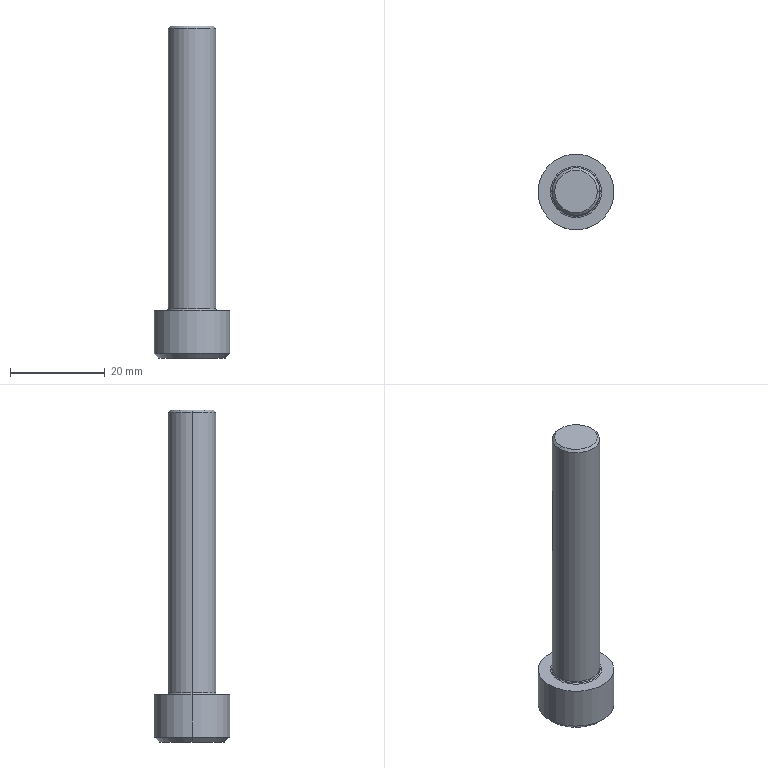Part | Creo | 1 solid | 23 faces | box 16 x 16 x 70 mm | volume 6361 mm3 | plane 9 | cone 6 | cylinder 4 | torus 4 | commonest cylinder face diameters 10 x2 16 x2
STEP:
#1=CARTESIAN_POINT('',(-135.619,-45.005,39.5));
#2=VERTEX_POINT('',#1);
#3=CARTESIAN_POINT('',(-133.309,-41.005,39.5));
#4=VERTEX_POINT('',#3);
#5=CARTESIAN_POINT('',(-135.619,-45.005,39.5));
#6=CARTESIAN_POINT('',(-135.493,-44.787,39.573));
#7=CARTESIAN_POINT('',(-135.241,-44.35,39.701));
#8=CARTESIAN_POINT('',(-134.855,-43.682,39.827));
#9=CARTESIAN_POINT('',(-134.465,-43.007,39.872));
#10=CARTESIAN_POINT('',(-134.074,-42.329,39.828));
#11=CARTESIAN_POINT('',(-133.689,-41.662,39.701));
#12=CARTESIAN_POINT('',(-133.436,-41.223,39.573));
#13=CARTESIAN_POINT('',(-133.309,-41.005,39.5));
#14=B_SPLINE_CURVE_WITH_KNOTS('',3,(#5,#6,#7,#8,#9,#10,#11,#12,#13),.UNSPECIFIED.,.F.,.F.,(4,1,1,1,1,1,4),(0.,0.1667,0.3333,0.5,0.6667,0.8333,1.),.UNSPECIFIED.);
#15=EDGE_CURVE('',#2,#4,#14,.T.);
#16=ORIENTED_EDGE('',*,*,#15,.F.);
#17=CARTESIAN_POINT('',(-131.,-45.005,42.167));
#18=VERTEX_POINT('',#17);
#19=CARTESIAN_POINT('',(-131.,-45.005,42.167));
#20=DIRECTION('',(-0.866,0.,-0.5));
#21=VECTOR('',#20,5.333);
#22=LINE('',#19,#21);
#23=EDGE_CURVE('',#18,#2,#22,.T.);
#24=ORIENTED_EDGE('',*,*,#23,.F.);
#25=CARTESIAN_POINT('',(-126.381,-45.005,39.5));
#26=VERTEX_POINT('',#25);
#27=CARTESIAN_POINT('',(-131.,-45.005,42.167));
#28=DIRECTION('',(0.866,0.,-0.5));
#29=VECTOR('',#28,5.333);
#30=LINE('',#27,#29);
#31=EDGE_CURVE('',#18,#26,#30,.T.);
#32=ORIENTED_EDGE('',*,*,#31,.T.);
#33=CARTESIAN_POINT('',(-128.691,-41.005,39.5));
#34=VERTEX_POINT('',#33);
#35=CARTESIAN_POINT('',(-128.691,-41.005,39.5));
#36=CARTESIAN_POINT('',(-128.565,-41.222,39.573));
#37=CARTESIAN_POINT('',(-128.313,-41.659,39.701));
#38=CARTESIAN_POINT('',(-127.927,-42.328,39.827));
#39=CARTESIAN_POINT('',(-127.537,-43.003,39.872));
#40=CARTESIAN_POINT('',(-127.146,-43.68,39.828));
#41=CARTESIAN_POINT('',(-126.761,-44.348,39.701));
#42=CARTESIAN_POINT('',(-126.507,-44.786,39.573));
#43=CARTESIAN_POINT('',(-126.381,-45.005,39.5));
#44=B_SPLINE_CURVE_WITH_KNOTS('',3,(#35,#36,#37,#38,#39,#40,#41,#42,#43),.UNSPECIFIED.,.F.,.F.,(4,1,1,1,1,1,4),(0.,0.1667,0.3333,0.5,0.6667,0.8333,1.),.UNSPECIFIED.);
#45=EDGE_CURVE('',#34,#26,#44,.T.);
#46=ORIENTED_EDGE('',*,*,#45,.F.);
#47=CARTESIAN_POINT('',(-133.309,-41.005,39.5));
#48=CARTESIAN_POINT('',(-133.059,-41.005,39.572));
#49=CARTESIAN_POINT('',(-132.556,-41.005,39.7));
#50=CARTESIAN_POINT('',(-131.782,-41.005,39.827));
#51=CARTESIAN_POINT('',(-131.001,-41.005,39.872));
#52=CARTESIAN_POINT('',(-130.221,-41.005,39.828));
#53=CARTESIAN_POINT('',(-129.447,-41.005,39.701));
#54=CARTESIAN_POINT('',(-128.942,-41.005,39.573));
#55=CARTESIAN_POINT('',(-128.691,-41.005,39.5));
#56=B_SPLINE_CURVE_WITH_KNOTS('',3,(#47,#48,#49,#50,#51,#52,#53,#54,#55),.UNSPECIFIED.,.F.,.F.,(4,1,1,1,1,1,4),(0.,0.1667,0.3333,0.5,0.6667,0.8333,1.),.UNSPECIFIED.);
#57=EDGE_CURVE('',#4,#34,#56,.T.);
#58=ORIENTED_EDGE('',*,*,#57,.F.);
#59=EDGE_LOOP('',(#16,#24,#32,#46,#58));
#60=FACE_OUTER_BOUND('',#59,.F.);
#61=CARTESIAN_POINT('',(-131.,-45.005,40.807));
#62=DIRECTION('',(0.,0.,-1.));
#63=DIRECTION('',(-1.,0.,0.));
#64=AXIS2_PLACEMENT_3D('',#61,#62,#63);
#65=CONICAL_SURFACE('',#64,2.356,60.);
#66=ADVANCED_FACE('',(#60),#65,.F.);
#67=CARTESIAN_POINT('',(-133.309,-41.005,34.5));
#68=VERTEX_POINT('',#67);
#69=CARTESIAN_POINT('',(-135.619,-45.005,34.5));
#70=VERTEX_POINT('',#69);
#71=CARTESIAN_POINT('',(-133.309,-41.005,34.5));
#72=DIRECTION('',(-0.5,-0.866,0.));
#73=VECTOR('',#72,4.619);
#74=LINE('',#71,#73);
#75=EDGE_CURVE('',#68,#70,#74,.T.);
#76=ORIENTED_EDGE('',*,*,#75,.T.);
#77=CARTESIAN_POINT('',(-135.619,-45.005,34.5));
#78=DIRECTION('',(0.,0.,1.));
#79=VECTOR('',#78,5.);
#80=LINE('',#77,#79);
#81=EDGE_CURVE('',#70,#2,#80,.T.);
#82=ORIENTED_EDGE('',*,*,#81,.T.);
#83=ORIENTED_EDGE('',*,*,#15,.T.);
#84=CARTESIAN_POINT('',(-133.309,-41.005,34.5));
#85=DIRECTION('',(0.,0.,1.));
#86=VECTOR('',#85,5.);
#87=LINE('',#84,#86);
#88=EDGE_CURVE('',#68,#4,#87,.T.);
#89=ORIENTED_EDGE('',*,*,#88,.F.);
#90=EDGE_LOOP('',(#76,#82,#83,#89));
#91=FACE_OUTER_BOUND('',#90,.F.);
#92=CARTESIAN_POINT('',(-133.309,-41.005,39.5));
#93=DIRECTION('',(0.866,-0.5,0.));
#94=DIRECTION('',(-0.5,-0.866,0.));
#95=AXIS2_PLACEMENT_3D('',#92,#93,#94);
#96=PLANE('',#95);
#97=ADVANCED_FACE('',(#91),#96,.T.);
#98=CARTESIAN_POINT('',(-138.,-45.005,34.5));
#99=VERTEX_POINT('',#98);
#100=CARTESIAN_POINT('',(-124.,-45.005,34.5));
#101=VERTEX_POINT('',#100);
#102=CARTESIAN_POINT('',(-131.,-45.005,34.5));
#103=DIRECTION('',(0.,0.,-1.));
#104=DIRECTION('',(-1.,0.,0.));
#105=AXIS2_PLACEMENT_3D('',#102,#103,#104);
#106=CIRCLE('',#105,7.);
#107=EDGE_CURVE('',#99,#101,#106,.T.);
#108=ORIENTED_EDGE('',*,*,#107,.F.);
#109=CARTESIAN_POINT('',(-131.,-45.005,34.5));
#110=DIRECTION('',(0.,0.,-1.));
#111=DIRECTION('',(1.,0.,0.));
#112=AXIS2_PLACEMENT_3D('',#109,#110,#111);
#113=CIRCLE('',#112,7.);
#114=EDGE_CURVE('',#101,#99,#113,.T.);
#115=ORIENTED_EDGE('',*,*,#114,.F.);
#116=EDGE_LOOP('',(#108,#115));
#117=FACE_OUTER_BOUND('',#116,.F.);
#118=CARTESIAN_POINT('',(-133.309,-49.005,34.5));
#119=VERTEX_POINT('',#118);
#120=CARTESIAN_POINT('',(-135.619,-45.005,34.5));
#121=DIRECTION('',(0.5,-0.866,0.));
#122=VECTOR('',#121,4.619);
#123=LINE('',#120,#122);
#124=EDGE_CURVE('',#70,#119,#123,.T.);
#125=ORIENTED_EDGE('',*,*,#124,.F.);
#126=ORIENTED_EDGE('',*,*,#75,.F.);
#127=CARTESIAN_POINT('',(-128.691,-41.005,34.5));
#128=VERTEX_POINT('',#127);
#129=CARTESIAN_POINT('',(-133.309,-41.005,34.5));
#130=DIRECTION('',(1.,0.,0.));
#131=VECTOR('',#130,4.619);
#132=LINE('',#129,#131);
#133=EDGE_CURVE('',#68,#128,#132,.T.);
#134=ORIENTED_EDGE('',*,*,#133,.T.);
#135=CARTESIAN_POINT('',(-126.381,-45.005,34.5));
#136=VERTEX_POINT('',#135);
#137=CARTESIAN_POINT('',(-126.381,-45.005,34.5));
#138=DIRECTION('',(-0.5,0.866,0.));
#139=VECTOR('',#138,4.619);
#140=LINE('',#137,#139);
#141=EDGE_CURVE('',#136,#128,#140,.T.);
#142=ORIENTED_EDGE('',*,*,#141,.F.);
#143=CARTESIAN_POINT('',(-128.691,-49.005,34.5));
#144=VERTEX_POINT('',#143);
#145=CARTESIAN_POINT('',(-128.691,-49.005,34.5));
#146=DIRECTION('',(0.5,0.866,0.));
#147=VECTOR('',#146,4.619);
#148=LINE('',#145,#147);
#149=EDGE_CURVE('',#144,#136,#148,.T.);
#150=ORIENTED_EDGE('',*,*,#149,.F.);
#151=CARTESIAN_POINT('',(-128.691,-49.005,34.5));
#152=DIRECTION('',(-1.,0.,0.));
#153=VECTOR('',#152,4.619);
#154=LINE('',#151,#153);
#155=EDGE_CURVE('',#144,#119,#154,.T.);
#156=ORIENTED_EDGE('',*,*,#155,.T.);
#157=EDGE_LOOP('',(#125,#126,#134,#142,#150,#156));
#158=FACE_BOUND('',#157,.F.);
#159=CARTESIAN_POINT('',(-131.,-45.005,34.5));
#160=DIRECTION('',(0.,0.,-1.));
#161=DIRECTION('',(-1.,0.,0.));
#162=AXIS2_PLACEMENT_3D('',#159,#160,#161);
#163=PLANE('',#162);
#164=ADVANCED_FACE('',(#117,#158),#163,.T.);
#165=CARTESIAN_POINT('',(-139.,-45.005,35.5));
#166=VERTEX_POINT('',#165);
#167=CARTESIAN_POINT('',(-123.,-45.005,35.5));
#168=VERTEX_POINT('',#167);
#169=CARTESIAN_POINT('',(-131.,-45.005,35.5));
#170=DIRECTION('',(0.,0.,-1.));
#171=DIRECTION('',(-1.,0.,0.));
#172=AXIS2_PLACEMENT_3D('',#169,#170,#171);
#173=CIRCLE('',#172,8.);
#174=EDGE_CURVE('',#166,#168,#173,.T.);
#175=ORIENTED_EDGE('',*,*,#174,.F.);
#176=CARTESIAN_POINT('',(-138.,-45.005,34.5));
#177=DIRECTION('',(-0.7071,0.,0.7071));
#178=VECTOR('',#177,1.414);
#179=LINE('',#176,#178);
#180=EDGE_CURVE('',#99,#166,#179,.T.);
#181=ORIENTED_EDGE('',*,*,#180,.F.);
#182=ORIENTED_EDGE('',*,*,#107,.T.);
#183=CARTESIAN_POINT('',(-124.,-45.005,34.5));
#184=DIRECTION('',(0.7071,0.,0.7071));
#185=VECTOR('',#184,1.414);
#186=LINE('',#183,#185);
#187=EDGE_CURVE('',#101,#168,#186,.T.);
#188=ORIENTED_EDGE('',*,*,#187,.T.);
#189=EDGE_LOOP('',(#175,#181,#182,#188));
#190=FACE_OUTER_BOUND('',#189,.F.);
#191=CARTESIAN_POINT('',(-131.,-45.005,35.));
#192=DIRECTION('',(0.,0.,1.));
#193=DIRECTION('',(1.,0.,0.));
#194=AXIS2_PLACEMENT_3D('',#191,#192,#193);
#195=CONICAL_SURFACE('',#194,7.5,45.);
#196=ADVANCED_FACE('',(#190),#195,.T.);
#197=ORIENTED_EDGE('',*,*,#174,.T.);
#198=CARTESIAN_POINT('',(-123.,-45.005,44.5));
#199=VERTEX_POINT('',#198);
#200=CARTESIAN_POINT('',(-123.,-45.005,44.5));
#201=DIRECTION('',(0.,0.,-1.));
#202=VECTOR('',#201,9.);
#203=LINE('',#200,#202);
#204=EDGE_CURVE('',#199,#168,#203,.T.);
#205=ORIENTED_EDGE('',*,*,#204,.F.);
#206=CARTESIAN_POINT('',(-139.,-45.005,44.5));
#207=VERTEX_POINT('',#206);
#208=CARTESIAN_POINT('',(-131.,-45.005,44.5));
#209=DIRECTION('',(0.,0.,1.));
#210=DIRECTION('',(1.,0.,0.));
#211=AXIS2_PLACEMENT_3D('',#208,#209,#210);
#212=CIRCLE('',#211,8.);
#213=EDGE_CURVE('',#199,#207,#212,.T.);
#214=ORIENTED_EDGE('',*,*,#213,.T.);
#215=CARTESIAN_POINT('',(-139.,-45.005,44.5));
#216=DIRECTION('',(0.,0.,-1.));
#217=VECTOR('',#216,9.);
#218=LINE('',#215,#217);
#219=EDGE_CURVE('',#207,#166,#218,.T.);
#220=ORIENTED_EDGE('',*,*,#219,.T.);
#221=EDGE_LOOP('',(#197,#205,#214,#220));
#222=FACE_OUTER_BOUND('',#221,.F.);
#223=CARTESIAN_POINT('',(-131.,-45.005,44.5));
#224=DIRECTION('',(0.,0.,-1.));
#225=DIRECTION('',(-1.,0.,0.));
#226=AXIS2_PLACEMENT_3D('',#223,#224,#225);
#227=CYLINDRICAL_SURFACE('',#226,8.);
#228=ADVANCED_FACE('',(#222),#227,.T.);
#229=CARTESIAN_POINT('',(-131.,-45.005,35.5));
#230=DIRECTION('',(0.,0.,-1.));
#231=DIRECTION('',(1.,0.,0.));
#232=AXIS2_PLACEMENT_3D('',#229,#230,#231);
#233=CIRCLE('',#232,8.);
#234=EDGE_CURVE('',#168,#166,#233,.T.);
#235=ORIENTED_EDGE('',*,*,#234,.T.);
#236=ORIENTED_EDGE('',*,*,#219,.F.);
#237=CARTESIAN_POINT('',(-131.,-45.005,44.5));
#238=DIRECTION('',(0.,0.,1.));
#239=DIRECTION('',(-1.,0.,0.));
#240=AXIS2_PLACEMENT_3D('',#237,#238,#239);
#241=CIRCLE('',#240,8.);
#242=EDGE_CURVE('',#207,#199,#241,.T.);
#243=ORIENTED_EDGE('',*,*,#242,.T.);
#244=ORIENTED_EDGE('',*,*,#204,.T.);
#245=EDGE_LOOP('',(#235,#236,#243,#244));
#246=FACE_OUTER_BOUND('',#245,.F.);
#247=CARTESIAN_POINT('',(-131.,-45.005,44.5));
#248=DIRECTION('',(0.,0.,-1.));
#249=DIRECTION('',(-1.,0.,0.));
#250=AXIS2_PLACEMENT_3D('',#247,#248,#249);
#251=CYLINDRICAL_SURFACE('',#250,8.);
#252=ADVANCED_FACE('',(#246),#251,.T.);
#253=ORIENTED_EDGE('',*,*,#234,.F.);
#254=ORIENTED_EDGE('',*,*,#187,.F.);
#255=ORIENTED_EDGE('',*,*,#114,.T.);
#256=ORIENTED_EDGE('',*,*,#180,.T.);
#257=EDGE_LOOP('',(#253,#254,#255,#256));
#258=FACE_OUTER_BOUND('',#257,.F.);
#259=CARTESIAN_POINT('',(-131.,-45.005,35.));
#260=DIRECTION('',(0.,0.,1.));
#261=DIRECTION('',(1.,0.,0.));
#262=AXIS2_PLACEMENT_3D('',#259,#260,#261);
#263=CONICAL_SURFACE('',#262,7.5,45.);
#264=ADVANCED_FACE('',(#258),#263,.T.);
#265=ORIENTED_EDGE('',*,*,#242,.F.);
#266=ORIENTED_EDGE('',*,*,#213,.F.);
#267=EDGE_LOOP('',(#265,#266));
#268=FACE_OUTER_BOUND('',#267,.F.);
#269=CARTESIAN_POINT('',(-136.4,-45.005,44.5));
#270=VERTEX_POINT('',#269);
#271=CARTESIAN_POINT('',(-125.6,-45.005,44.5));
#272=VERTEX_POINT('',#271);
#273=CARTESIAN_POINT('',(-131.,-45.005,44.5));
#274=DIRECTION('',(0.,0.,-1.));
#275=DIRECTION('',(-1.,0.,0.));
#276=AXIS2_PLACEMENT_3D('',#273,#274,#275);
#277=CIRCLE('',#276,5.4);
#278=EDGE_CURVE('',#270,#272,#277,.T.);
#279=ORIENTED_EDGE('',*,*,#278,.F.);
#280=CARTESIAN_POINT('',(-131.,-45.005,44.5));
#281=DIRECTION('',(0.,0.,-1.));
#282=DIRECTION('',(1.,0.,0.));
#283=AXIS2_PLACEMENT_3D('',#280,#281,#282);
#284=CIRCLE('',#283,5.4);
#285=EDGE_CURVE('',#272,#270,#284,.T.);
#286=ORIENTED_EDGE('',*,*,#285,.F.);
#287=EDGE_LOOP('',(#279,#286));
#288=FACE_BOUND('',#287,.F.);
#289=CARTESIAN_POINT('',(-131.,-45.005,44.5));
#290=DIRECTION('',(0.,0.,-1.));
#291=DIRECTION('',(-1.,0.,0.));
#292=AXIS2_PLACEMENT_3D('',#289,#290,#291);
#293=PLANE('',#292);
#294=ADVANCED_FACE('',(#268,#288),#293,.F.);
#295=ORIENTED_EDGE('',*,*,#278,.T.);
#296=CARTESIAN_POINT('',(-125.883,-45.005,44.617));
#297=VERTEX_POINT('',#296);
#298=CARTESIAN_POINT('',(-125.6,-45.005,44.9));
#299=DIRECTION('',(0.,1.,0.));
#300=DIRECTION('',(0.,0.,-1.));
#301=AXIS2_PLACEMENT_3D('',#298,#299,#300);
#302=CIRCLE('',#301,0.4);
#303=EDGE_CURVE('',#272,#297,#302,.T.);
#304=ORIENTED_EDGE('',*,*,#303,.T.);
#305=CARTESIAN_POINT('',(-136.117,-45.005,44.617));
#306=VERTEX_POINT('',#305);
#307=CARTESIAN_POINT('',(-131.,-45.005,44.617));
#308=DIRECTION('',(0.,0.,-1.));
#309=DIRECTION('',(-1.,0.,0.));
#310=AXIS2_PLACEMENT_3D('',#307,#308,#309);
#311=CIRCLE('',#310,5.117);
#312=EDGE_CURVE('',#306,#297,#311,.T.);
#313=ORIENTED_EDGE('',*,*,#312,.F.);
#314=CARTESIAN_POINT('',(-136.4,-45.005,44.9));
#315=DIRECTION('',(0.,-1.,0.));
#316=DIRECTION('',(0.,0.,-1.));
#317=AXIS2_PLACEMENT_3D('',#314,#315,#316);
#318=CIRCLE('',#317,0.4);
#319=EDGE_CURVE('',#270,#306,#318,.T.);
#320=ORIENTED_EDGE('',*,*,#319,.F.);
#321=EDGE_LOOP('',(#295,#304,#313,#320));
#322=FACE_OUTER_BOUND('',#321,.F.);
#323=CARTESIAN_POINT('',(-131.,-45.005,44.9));
#324=DIRECTION('',(0.,0.,-1.));
#325=DIRECTION('',(-1.,0.,0.));
#326=AXIS2_PLACEMENT_3D('',#323,#324,#325);
#327=TOROIDAL_SURFACE('',#326,5.4,0.4);
#328=ADVANCED_FACE('',(#322),#327,.F.);
#329=ORIENTED_EDGE('',*,*,#285,.T.);
#330=ORIENTED_EDGE('',*,*,#319,.T.);
#331=CARTESIAN_POINT('',(-131.,-45.005,44.617));
#332=DIRECTION('',(0.,0.,-1.));
#333=DIRECTION('',(1.,0.,0.));
#334=AXIS2_PLACEMENT_3D('',#331,#332,#333);
#335=CIRCLE('',#334,5.117);
#336=EDGE_CURVE('',#297,#306,#335,.T.);
#337=ORIENTED_EDGE('',*,*,#336,.F.);
#338=ORIENTED_EDGE('',*,*,#303,.F.);
#339=EDGE_LOOP('',(#329,#330,#337,#338));
#340=FACE_OUTER_BOUND('',#339,.F.);
#341=CARTESIAN_POINT('',(-131.,-45.005,44.9));
#342=DIRECTION('',(0.,0.,-1.));
#343=DIRECTION('',(-1.,0.,0.));
#344=AXIS2_PLACEMENT_3D('',#341,#342,#343);
#345=TOROIDAL_SURFACE('',#344,5.4,0.4);
#346=ADVANCED_FACE('',(#340),#345,.F.);
#347=CARTESIAN_POINT('',(-126.,-45.005,44.9));
#348=VERTEX_POINT('',#347);
#349=CARTESIAN_POINT('',(-136.,-45.005,44.9));
#350=VERTEX_POINT('',#349);
#351=CARTESIAN_POINT('',(-131.,-45.005,44.9));
#352=DIRECTION('',(0.,0.,-1.));
#353=DIRECTION('',(1.,0.,0.));
#354=AXIS2_PLACEMENT_3D('',#351,#352,#353);
#355=CIRCLE('',#354,5.);
#356=EDGE_CURVE('',#348,#350,#355,.T.);
#357=ORIENTED_EDGE('',*,*,#356,.F.);
#358=CARTESIAN_POINT('',(-125.6,-45.005,44.9));
#359=DIRECTION('',(0.,1.,0.));
#360=DIRECTION('',(-0.7071,0.,-0.7071));
#361=AXIS2_PLACEMENT_3D('',#358,#359,#360);
#362=CIRCLE('',#361,0.4);
#363=EDGE_CURVE('',#297,#348,#362,.T.);
#364=ORIENTED_EDGE('',*,*,#363,.F.);
#365=ORIENTED_EDGE('',*,*,#336,.T.);
#366=CARTESIAN_POINT('',(-136.4,-45.005,44.9));
#367=DIRECTION('',(0.,-1.,0.));
#368=DIRECTION('',(0.7071,0.,-0.7071));
#369=AXIS2_PLACEMENT_3D('',#366,#367,#368);
#370=CIRCLE('',#369,0.4);
#371=EDGE_CURVE('',#306,#350,#370,.T.);
#372=ORIENTED_EDGE('',*,*,#371,.T.);
#373=EDGE_LOOP('',(#357,#364,#365,#372));
#374=FACE_OUTER_BOUND('',#373,.F.);
#375=CARTESIAN_POINT('',(-131.,-45.005,44.9));
#376=DIRECTION('',(0.,0.,-1.));
#377=DIRECTION('',(-1.,0.,0.));
#378=AXIS2_PLACEMENT_3D('',#375,#376,#377);
#379=TOROIDAL_SURFACE('',#378,5.4,0.4);
#380=ADVANCED_FACE('',(#374),#379,.F.);
#381=CARTESIAN_POINT('',(-136.,-45.005,104.));
#382=VERTEX_POINT('',#381);
#383=CARTESIAN_POINT('',(-126.,-45.005,104.));
#384=VERTEX_POINT('',#383);
#385=CARTESIAN_POINT('',(-131.,-45.005,104.));
#386=DIRECTION('',(0.,0.,1.));
#387=DIRECTION('',(-1.,0.,0.));
#388=AXIS2_PLACEMENT_3D('',#385,#386,#387);
#389=CIRCLE('',#388,5.);
#390=EDGE_CURVE('',#382,#384,#389,.T.);
#391=ORIENTED_EDGE('',*,*,#390,.T.);
#392=CARTESIAN_POINT('',(-126.,-45.005,104.));
#393=DIRECTION('',(0.,0.,-1.));
#394=VECTOR('',#393,59.1);
#395=LINE('',#392,#394);
#396=EDGE_CURVE('',#384,#348,#395,.T.);
#397=ORIENTED_EDGE('',*,*,#396,.T.);
#398=ORIENTED_EDGE('',*,*,#356,.T.);
#399=CARTESIAN_POINT('',(-136.,-45.005,104.));
#400=DIRECTION('',(0.,0.,-1.));
#401=VECTOR('',#400,59.1);
#402=LINE('',#399,#401);
#403=EDGE_CURVE('',#382,#350,#402,.T.);
#404=ORIENTED_EDGE('',*,*,#403,.F.);
#405=EDGE_LOOP('',(#391,#397,#398,#404));
#406=FACE_OUTER_BOUND('',#405,.F.);
#407=CARTESIAN_POINT('',(-131.,-45.005,104.5));
#408=DIRECTION('',(0.,0.,-1.));
#409=DIRECTION('',(-1.,0.,0.));
#410=AXIS2_PLACEMENT_3D('',#407,#408,#409);
#411=CYLINDRICAL_SURFACE('',#410,5.);
#412=ADVANCED_FACE('',(#406),#411,.T.);
#413=CARTESIAN_POINT('',(-135.5,-45.005,104.5));
#414=VERTEX_POINT('',#413);
#415=CARTESIAN_POINT('',(-126.5,-45.005,104.5));
#416=VERTEX_POINT('',#415);
#417=CARTESIAN_POINT('',(-131.,-45.005,104.5));
#418=DIRECTION('',(0.,0.,1.));
#419=DIRECTION('',(-1.,0.,0.));
#420=AXIS2_PLACEMENT_3D('',#417,#418,#419);
#421=CIRCLE('',#420,4.5);
#422=EDGE_CURVE('',#414,#416,#421,.T.);
#423=ORIENTED_EDGE('',*,*,#422,.T.);
#424=CARTESIAN_POINT('',(-126.5,-45.005,104.5));
#425=DIRECTION('',(0.7071,0.,-0.7071));
#426=VECTOR('',#425,0.7071);
#427=LINE('',#424,#426);
#428=EDGE_CURVE('',#416,#384,#427,.T.);
#429=ORIENTED_EDGE('',*,*,#428,.T.);
#430=ORIENTED_EDGE('',*,*,#390,.F.);
#431=CARTESIAN_POINT('',(-135.5,-45.005,104.5));
#432=DIRECTION('',(-0.7071,0.,-0.7071));
#433=VECTOR('',#432,0.7071);
#434=LINE('',#431,#433);
#435=EDGE_CURVE('',#414,#382,#434,.T.);
#436=ORIENTED_EDGE('',*,*,#435,.F.);
#437=EDGE_LOOP('',(#423,#429,#430,#436));
#438=FACE_OUTER_BOUND('',#437,.F.);
#439=CARTESIAN_POINT('',(-131.,-45.005,104.25));
#440=DIRECTION('',(0.,0.,-1.));
#441=DIRECTION('',(-1.,0.,0.));
#442=AXIS2_PLACEMENT_3D('',#439,#440,#441);
#443=CONICAL_SURFACE('',#442,4.75,45.);
#444=ADVANCED_FACE('',(#438),#443,.T.);
#445=ORIENTED_EDGE('',*,*,#422,.F.);
#446=CARTESIAN_POINT('',(-131.,-45.005,104.5));
#447=DIRECTION('',(0.,0.,1.));
#448=DIRECTION('',(1.,0.,0.));
#449=AXIS2_PLACEMENT_3D('',#446,#447,#448);
#450=CIRCLE('',#449,4.5);
#451=EDGE_CURVE('',#416,#414,#450,.T.);
#452=ORIENTED_EDGE('',*,*,#451,.F.);
#453=EDGE_LOOP('',(#445,#452));
#454=FACE_OUTER_BOUND('',#453,.F.);
#455=CARTESIAN_POINT('',(-131.,-45.005,104.5));
#456=DIRECTION('',(0.,0.,-1.));
#457=DIRECTION('',(-1.,0.,0.));
#458=AXIS2_PLACEMENT_3D('',#455,#456,#457);
#459=PLANE('',#458);
#460=ADVANCED_FACE('',(#454),#459,.F.);
#461=ORIENTED_EDGE('',*,*,#451,.T.);
#462=ORIENTED_EDGE('',*,*,#435,.T.);
#463=CARTESIAN_POINT('',(-131.,-45.005,104.));
#464=DIRECTION('',(0.,0.,1.));
#465=DIRECTION('',(1.,0.,0.));
#466=AXIS2_PLACEMENT_3D('',#463,#464,#465);
#467=CIRCLE('',#466,5.);
#468=EDGE_CURVE('',#384,#382,#467,.T.);
#469=ORIENTED_EDGE('',*,*,#468,.F.);
#470=ORIENTED_EDGE('',*,*,#428,.F.);
#471=EDGE_LOOP('',(#461,#462,#469,#470));
#472=FACE_OUTER_BOUND('',#471,.F.);
#473=CARTESIAN_POINT('',(-131.,-45.005,104.25));
#474=DIRECTION('',(0.,0.,-1.));
#475=DIRECTION('',(-1.,0.,0.));
#476=AXIS2_PLACEMENT_3D('',#473,#474,#475);
#477=CONICAL_SURFACE('',#476,4.75,45.);
#478=ADVANCED_FACE('',(#472),#477,.T.);
#479=ORIENTED_EDGE('',*,*,#468,.T.);
#480=ORIENTED_EDGE('',*,*,#403,.T.);
#481=CARTESIAN_POINT('',(-131.,-45.005,44.9));
#482=DIRECTION('',(0.,0.,-1.));
#483=DIRECTION('',(-1.,0.,0.));
#484=AXIS2_PLACEMENT_3D('',#481,#482,#483);
#485=CIRCLE('',#484,5.);
#486=EDGE_CURVE('',#350,#348,#485,.T.);
#487=ORIENTED_EDGE('',*,*,#486,.T.);
#488=ORIENTED_EDGE('',*,*,#396,.F.);
#489=EDGE_LOOP('',(#479,#480,#487,#488));
#490=FACE_OUTER_BOUND('',#489,.F.);
#491=CARTESIAN_POINT('',(-131.,-45.005,104.5));
#492=DIRECTION('',(0.,0.,-1.));
#493=DIRECTION('',(-1.,0.,0.));
#494=AXIS2_PLACEMENT_3D('',#491,#492,#493);
#495=CYLINDRICAL_SURFACE('',#494,5.);
#496=ADVANCED_FACE('',(#490),#495,.T.);
#497=ORIENTED_EDGE('',*,*,#486,.F.);
#498=ORIENTED_EDGE('',*,*,#371,.F.);
#499=ORIENTED_EDGE('',*,*,#312,.T.);
#500=ORIENTED_EDGE('',*,*,#363,.T.);
#501=EDGE_LOOP('',(#497,#498,#499,#500));
#502=FACE_OUTER_BOUND('',#501,.F.);
#503=CARTESIAN_POINT('',(-131.,-45.005,44.9));
#504=DIRECTION('',(0.,0.,-1.));
#505=DIRECTION('',(-1.,0.,0.));
#506=AXIS2_PLACEMENT_3D('',#503,#504,#505);
#507=TOROIDAL_SURFACE('',#506,5.4,0.4);
#508=ADVANCED_FACE('',(#502),#507,.F.);
#509=ORIENTED_EDGE('',*,*,#124,.T.);
#510=CARTESIAN_POINT('',(-133.309,-49.005,39.5));
#511=VERTEX_POINT('',#510);
#512=CARTESIAN_POINT('',(-133.309,-49.005,34.5));
#513=DIRECTION('',(0.,0.,1.));
#514=VECTOR('',#513,5.);
#515=LINE('',#512,#514);
#516=EDGE_CURVE('',#119,#511,#515,.T.);
#517=ORIENTED_EDGE('',*,*,#516,.T.);
#518=CARTESIAN_POINT('',(-133.309,-49.005,39.5));
#519=CARTESIAN_POINT('',(-133.435,-48.787,39.573));
#520=CARTESIAN_POINT('',(-133.687,-48.35,39.701));
#521=CARTESIAN_POINT('',(-134.073,-47.682,39.827));
#522=CARTESIAN_POINT('',(-134.463,-47.007,39.872));
#523=CARTESIAN_POINT('',(-134.854,-46.329,39.828));
#524=CARTESIAN_POINT('',(-135.239,-45.662,39.701));
#525=CARTESIAN_POINT('',(-135.493,-45.223,39.573));
#526=CARTESIAN_POINT('',(-135.619,-45.005,39.5));
#527=B_SPLINE_CURVE_WITH_KNOTS('',3,(#518,#519,#520,#521,#522,#523,#524,#525,#526),.UNSPECIFIED.,.F.,.F.,(4,1,1,1,1,1,4),(0.,0.1667,0.3333,0.5,0.6667,0.8333,1.),.UNSPECIFIED.);
#528=EDGE_CURVE('',#511,#2,#527,.T.);
#529=ORIENTED_EDGE('',*,*,#528,.T.);
#530=ORIENTED_EDGE('',*,*,#81,.F.);
#531=EDGE_LOOP('',(#509,#517,#529,#530));
#532=FACE_OUTER_BOUND('',#531,.F.);
#533=CARTESIAN_POINT('',(-135.619,-45.005,39.5));
#534=DIRECTION('',(0.866,0.5,0.));
#535=DIRECTION('',(0.5,-0.866,0.));
#536=AXIS2_PLACEMENT_3D('',#533,#534,#535);
#537=PLANE('',#536);
#538=ADVANCED_FACE('',(#532),#537,.T.);
#539=ORIENTED_EDGE('',*,*,#155,.F.);
#540=CARTESIAN_POINT('',(-128.691,-49.005,39.5));
#541=VERTEX_POINT('',#540);
#542=CARTESIAN_POINT('',(-128.691,-49.005,34.5));
#543=DIRECTION('',(0.,0.,1.));
#544=VECTOR('',#543,5.);
#545=LINE('',#542,#544);
#546=EDGE_CURVE('',#144,#541,#545,.T.);
#547=ORIENTED_EDGE('',*,*,#546,.T.);
#548=CARTESIAN_POINT('',(-128.691,-49.005,39.5));
#549=CARTESIAN_POINT('',(-128.942,-49.005,39.573));
#550=CARTESIAN_POINT('',(-129.447,-49.005,39.701));
#551=CARTESIAN_POINT('',(-130.221,-49.005,39.828));
#552=CARTESIAN_POINT('',(-131.001,-49.005,39.872));
#553=CARTESIAN_POINT('',(-131.782,-49.005,39.827));
#554=CARTESIAN_POINT('',(-132.556,-49.005,39.7));
#555=CARTESIAN_POINT('',(-133.059,-49.005,39.572));
#556=CARTESIAN_POINT('',(-133.309,-49.005,39.5));
#557=B_SPLINE_CURVE_WITH_KNOTS('',3,(#548,#549,#550,#551,#552,#553,#554,#555,#556),.UNSPECIFIED.,.F.,.F.,(4,1,1,1,1,1,4),(0.,0.1667,0.3333,0.5,0.6667,0.8333,1.),.UNSPECIFIED.);
#558=EDGE_CURVE('',#541,#511,#557,.T.);
#559=ORIENTED_EDGE('',*,*,#558,.T.);
#560=ORIENTED_EDGE('',*,*,#516,.F.);
#561=EDGE_LOOP('',(#539,#547,#559,#560));
#562=FACE_OUTER_BOUND('',#561,.F.);
#563=CARTESIAN_POINT('',(-133.309,-49.005,39.5));
#564=DIRECTION('',(0.,1.,0.));
#565=DIRECTION('',(0.,0.,-1.));
#566=AXIS2_PLACEMENT_3D('',#563,#564,#565);
#567=PLANE('',#566);
#568=ADVANCED_FACE('',(#562),#567,.T.);
#569=ORIENTED_EDGE('',*,*,#149,.T.);
#570=CARTESIAN_POINT('',(-126.381,-45.005,34.5));
#571=DIRECTION('',(0.,0.,1.));
#572=VECTOR('',#571,5.);
#573=LINE('',#570,#572);
#574=EDGE_CURVE('',#136,#26,#573,.T.);
#575=ORIENTED_EDGE('',*,*,#574,.T.);
#576=CARTESIAN_POINT('',(-126.381,-45.005,39.5));
#577=CARTESIAN_POINT('',(-126.507,-45.223,39.573));
#578=CARTESIAN_POINT('',(-126.761,-45.662,39.701));
#579=CARTESIAN_POINT('',(-127.146,-46.329,39.828));
#580=CARTESIAN_POINT('',(-127.537,-47.007,39.872));
#581=CARTESIAN_POINT('',(-127.927,-47.682,39.827));
#582=CARTESIAN_POINT('',(-128.313,-48.35,39.701));
#583=CARTESIAN_POINT('',(-128.565,-48.787,39.573));
#584=CARTESIAN_POINT('',(-128.691,-49.005,39.5));
#585=B_SPLINE_CURVE_WITH_KNOTS('',3,(#576,#577,#578,#579,#580,#581,#582,#583,#584),.UNSPECIFIED.,.F.,.F.,(4,1,1,1,1,1,4),(0.,0.1667,0.3333,0.5,0.6667,0.8333,1.),.UNSPECIFIED.);
#586=EDGE_CURVE('',#26,#541,#585,.T.);
#587=ORIENTED_EDGE('',*,*,#586,.T.);
#588=ORIENTED_EDGE('',*,*,#546,.F.);
#589=EDGE_LOOP('',(#569,#575,#587,#588));
#590=FACE_OUTER_BOUND('',#589,.F.);
#591=CARTESIAN_POINT('',(-128.691,-49.005,39.5));
#592=DIRECTION('',(-0.866,0.5,0.));
#593=DIRECTION('',(0.5,0.866,0.));
#594=AXIS2_PLACEMENT_3D('',#591,#592,#593);
#595=PLANE('',#594);
#596=ADVANCED_FACE('',(#590),#595,.T.);
#597=ORIENTED_EDGE('',*,*,#141,.T.);
#598=CARTESIAN_POINT('',(-128.691,-41.005,34.5));
#599=DIRECTION('',(0.,0.,1.));
#600=VECTOR('',#599,5.);
#601=LINE('',#598,#600);
#602=EDGE_CURVE('',#128,#34,#601,.T.);
#603=ORIENTED_EDGE('',*,*,#602,.T.);
#604=ORIENTED_EDGE('',*,*,#45,.T.);
#605=ORIENTED_EDGE('',*,*,#574,.F.);
#606=EDGE_LOOP('',(#597,#603,#604,#605));
#607=FACE_OUTER_BOUND('',#606,.F.);
#608=CARTESIAN_POINT('',(-126.381,-45.005,39.5));
#609=DIRECTION('',(-0.866,-0.5,0.));
#610=DIRECTION('',(-0.5,0.866,0.));
#611=AXIS2_PLACEMENT_3D('',#608,#609,#610);
#612=PLANE('',#611);
#613=ADVANCED_FACE('',(#607),#612,.T.);
#614=ORIENTED_EDGE('',*,*,#133,.F.);
#615=ORIENTED_EDGE('',*,*,#88,.T.);
#616=ORIENTED_EDGE('',*,*,#57,.T.);
#617=ORIENTED_EDGE('',*,*,#602,.F.);
#618=EDGE_LOOP('',(#614,#615,#616,#617));
#619=FACE_OUTER_BOUND('',#618,.F.);
#620=CARTESIAN_POINT('',(-128.691,-41.005,39.5));
#621=DIRECTION('',(0.,-1.,0.));
#622=DIRECTION('',(0.,0.,1.));
#623=AXIS2_PLACEMENT_3D('',#620,#621,#622);
#624=PLANE('',#623);
#625=ADVANCED_FACE('',(#619),#624,.T.);
#626=ORIENTED_EDGE('',*,*,#586,.F.);
#627=ORIENTED_EDGE('',*,*,#31,.F.);
#628=ORIENTED_EDGE('',*,*,#23,.T.);
#629=ORIENTED_EDGE('',*,*,#528,.F.);
#630=ORIENTED_EDGE('',*,*,#558,.F.);
#631=EDGE_LOOP('',(#626,#627,#628,#629,#630));
#632=FACE_OUTER_BOUND('',#631,.F.);
#633=CARTESIAN_POINT('',(-131.,-45.005,40.807));
#634=DIRECTION('',(0.,0.,-1.));
#635=DIRECTION('',(-1.,0.,0.));
#636=AXIS2_PLACEMENT_3D('',#633,#634,#635);
#637=CONICAL_SURFACE('',#636,2.356,60.);
#638=ADVANCED_FACE('',(#632),#637,.F.);
#639=CLOSED_SHELL('',(#66,#97,#164,#196,#228,#252,#264,#294,#328,#346,#380,#412,#444,#460,#478,#496,#508,#538,#568,#596,#613,#625,#638));
#640=MANIFOLD_SOLID_BREP('',#639);
#641=(LENGTH_UNIT()NAMED_UNIT(*)SI_UNIT(.MILLI.,.METRE.));
#642=UNCERTAINTY_MEASURE_WITH_UNIT(LENGTH_MEASURE(0.007357),#641,'','');
#643=(NAMED_UNIT(*)PLANE_ANGLE_UNIT()SI_UNIT($,.RADIAN.));
#644=PLANE_ANGLE_MEASURE_WITH_UNIT(PLANE_ANGLE_MEASURE(0.01745),#643);
#645=(CONVERSION_BASED_UNIT('DEGREE',#644)NAMED_UNIT(*)PLANE_ANGLE_UNIT());
#646=(NAMED_UNIT(*)SI_UNIT($,.STERADIAN.)SOLID_ANGLE_UNIT());
#647=(GEOMETRIC_REPRESENTATION_CONTEXT(3)GLOBAL_UNCERTAINTY_ASSIGNED_CONTEXT((#642))GLOBAL_UNIT_ASSIGNED_CONTEXT((#641,#645,#646))REPRESENTATION_CONTEXT('',''));
#648=ADVANCED_BREP_SHAPE_REPRESENTATION('',(#640),#647);